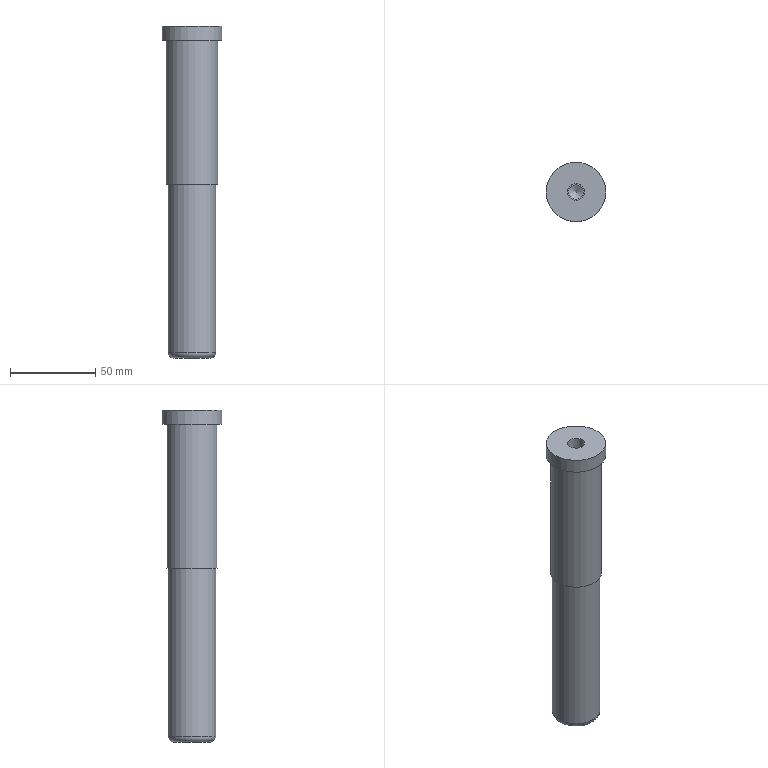Part | STEP file | solid 153 | 1 solid | 12 faces | box 35 x 35 x 195 mm | volume 128650 mm3 | plane 5 | cylinder 5 | cone 1 | torus 1 | commonest cylinder face diameters 8.5 x1 10 x1 28 x1 30 x1 35 x1